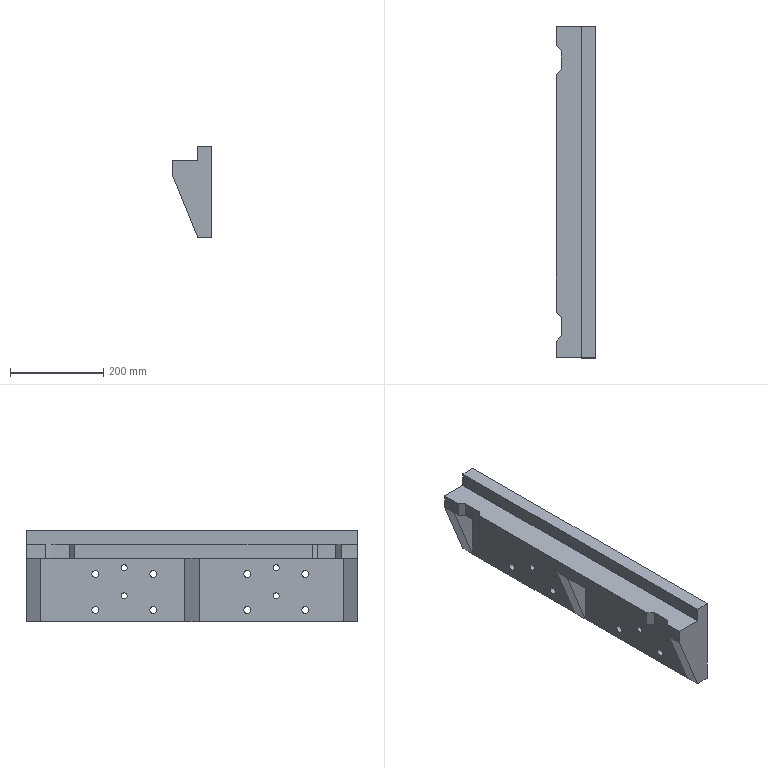Part | NX | features solid 2 | 1 solid | 39 faces | box 85 x 710 x 195 mm | volume 5567126 mm3 | plane 27 | cylinder 12 | commonest cylinder face diameters 15 x8 13 x4
STEP:
#1=CARTESIAN_POINT('',(780.,114.5,-108.));
#2=VERTEX_POINT('',#1);
#3=CARTESIAN_POINT('',(780.,107.,-108.));
#4=DIRECTION('',(1.,0.,0.));
#5=DIRECTION('',(0.,1.,0.));
#6=AXIS2_PLACEMENT_3D('',#3,#4,#5);
#7=CIRCLE('',#6,7.5);
#8=EDGE_CURVE('',#2,#2,#7,.F.);
#9=ORIENTED_EDGE('',*,*,#8,.F.);
#10=EDGE_LOOP('',(#9));
#11=FACE_BOUND('',#10,.T.);
#12=CARTESIAN_POINT('',(780.,114.5,-185.));
#13=VERTEX_POINT('',#12);
#14=CARTESIAN_POINT('',(780.,107.,-185.));
#15=DIRECTION('',(1.,0.,0.));
#16=DIRECTION('',(0.,1.,0.));
#17=AXIS2_PLACEMENT_3D('',#14,#15,#16);
#18=CIRCLE('',#17,7.5);
#19=EDGE_CURVE('',#13,#13,#18,.F.);
#20=ORIENTED_EDGE('',*,*,#19,.F.);
#21=EDGE_LOOP('',(#20));
#22=FACE_BOUND('',#21,.T.);
#23=CARTESIAN_POINT('',(780.,51.5,-155.));
#24=VERTEX_POINT('',#23);
#25=CARTESIAN_POINT('',(780.,45.,-155.));
#26=DIRECTION('',(1.,0.,0.));
#27=DIRECTION('',(0.,1.,0.));
#28=AXIS2_PLACEMENT_3D('',#25,#26,#27);
#29=CIRCLE('',#28,6.5);
#30=EDGE_CURVE('',#24,#24,#29,.T.);
#31=ORIENTED_EDGE('',*,*,#30,.T.);
#32=EDGE_LOOP('',(#31));
#33=FACE_BOUND('',#32,.T.);
#34=CARTESIAN_POINT('',(780.,-9.5,-185.));
#35=VERTEX_POINT('',#34);
#36=CARTESIAN_POINT('',(780.,-17.,-185.));
#37=DIRECTION('',(1.,0.,0.));
#38=DIRECTION('',(0.,1.,0.));
#39=AXIS2_PLACEMENT_3D('',#36,#37,#38);
#40=CIRCLE('',#39,7.5);
#41=EDGE_CURVE('',#35,#35,#40,.F.);
#42=ORIENTED_EDGE('',*,*,#41,.F.);
#43=EDGE_LOOP('',(#42));
#44=FACE_BOUND('',#43,.T.);
#45=CARTESIAN_POINT('',(780.,51.5,-95.));
#46=VERTEX_POINT('',#45);
#47=CARTESIAN_POINT('',(780.,45.,-95.));
#48=DIRECTION('',(1.,0.,0.));
#49=DIRECTION('',(0.,1.,0.));
#50=AXIS2_PLACEMENT_3D('',#47,#48,#49);
#51=CIRCLE('',#50,6.5);
#52=EDGE_CURVE('',#46,#46,#51,.T.);
#53=ORIENTED_EDGE('',*,*,#52,.T.);
#54=EDGE_LOOP('',(#53));
#55=FACE_BOUND('',#54,.T.);
#56=CARTESIAN_POINT('',(780.,-9.5,-108.));
#57=VERTEX_POINT('',#56);
#58=CARTESIAN_POINT('',(780.,-17.,-108.));
#59=DIRECTION('',(1.,0.,0.));
#60=DIRECTION('',(0.,1.,0.));
#61=AXIS2_PLACEMENT_3D('',#58,#59,#60);
#62=CIRCLE('',#61,7.5);
#63=EDGE_CURVE('',#57,#57,#62,.F.);
#64=ORIENTED_EDGE('',*,*,#63,.F.);
#65=EDGE_LOOP('',(#64));
#66=FACE_BOUND('',#65,.T.);
#67=CARTESIAN_POINT('',(780.,225.,-210.));
#68=VERTEX_POINT('',#67);
#69=CARTESIAN_POINT('',(780.,-85.,-210.));
#70=VERTEX_POINT('',#69);
#71=CARTESIAN_POINT('',(780.,-20.,-210.));
#72=DIRECTION('',(0.,1.,0.));
#73=VECTOR('',#72,1000.);
#74=LINE('',#71,#73);
#75=EDGE_CURVE('',#68,#70,#74,.F.);
#76=ORIENTED_EDGE('',*,*,#75,.T.);
#77=CARTESIAN_POINT('',(780.,-85.,-75.));
#78=VERTEX_POINT('',#77);
#79=CARTESIAN_POINT('',(780.,-85.,-75.));
#80=DIRECTION('',(0.,0.,-1.));
#81=VECTOR('',#80,1000.);
#82=LINE('',#79,#81);
#83=EDGE_CURVE('',#78,#70,#82,.T.);
#84=ORIENTED_EDGE('',*,*,#83,.F.);
#85=CARTESIAN_POINT('',(780.,225.,-75.));
#86=VERTEX_POINT('',#85);
#87=CARTESIAN_POINT('',(780.,-20.,-75.));
#88=DIRECTION('',(0.,1.,0.));
#89=VECTOR('',#88,1000.);
#90=LINE('',#87,#89);
#91=EDGE_CURVE('',#78,#86,#90,.T.);
#92=ORIENTED_EDGE('',*,*,#91,.T.);
#93=CARTESIAN_POINT('',(780.,225.,-75.));
#94=DIRECTION('',(0.,0.,-1.));
#95=VECTOR('',#94,1000.);
#96=LINE('',#93,#95);
#97=EDGE_CURVE('',#86,#68,#96,.T.);
#98=ORIENTED_EDGE('',*,*,#97,.T.);
#99=EDGE_LOOP('',(#76,#84,#92,#98));
#100=FACE_BOUND('',#99,.T.);
#101=CARTESIAN_POINT('',(780.,-330.,-15.974));
#102=DIRECTION('',(1.,0.,0.));
#103=DIRECTION('',(0.,1.,0.));
#104=AXIS2_PLACEMENT_3D('',#101,#102,#103);
#105=PLANE('',#104);
#106=ADVANCED_FACE('',(#11,#22,#33,#44,#55,#66,#100),#105,.F.);
#107=ORIENTED_EDGE('',*,*,#91,.F.);
#108=CARTESIAN_POINT('',(725.,-85.,-75.));
#109=VERTEX_POINT('',#108);
#110=CARTESIAN_POINT('',(780.,-85.,-75.));
#111=DIRECTION('',(-1.,0.,0.));
#112=VECTOR('',#111,1000.);
#113=LINE('',#110,#112);
#114=EDGE_CURVE('',#78,#109,#113,.T.);
#115=ORIENTED_EDGE('',*,*,#114,.T.);
#116=CARTESIAN_POINT('',(725.,151.,-75.));
#117=VERTEX_POINT('',#116);
#118=CARTESIAN_POINT('',(725.,-370.,-75.));
#119=DIRECTION('',(0.,-1.,0.));
#120=VECTOR('',#119,1000.);
#121=LINE('',#118,#120);
#122=EDGE_CURVE('',#117,#109,#121,.T.);
#123=ORIENTED_EDGE('',*,*,#122,.F.);
#124=CARTESIAN_POINT('',(736.,162.,-75.));
#125=VERTEX_POINT('',#124);
#126=CARTESIAN_POINT('',(842.,268.,-75.));
#127=DIRECTION('',(0.7071,0.7071,0.));
#128=VECTOR('',#127,1000.);
#129=LINE('',#126,#128);
#130=EDGE_CURVE('',#117,#125,#129,.T.);
#131=ORIENTED_EDGE('',*,*,#130,.T.);
#132=CARTESIAN_POINT('',(736.,202.,-75.));
#133=VERTEX_POINT('',#132);
#134=CARTESIAN_POINT('',(736.,330.,-75.));
#135=DIRECTION('',(0.,-1.,0.));
#136=VECTOR('',#135,1000.);
#137=LINE('',#134,#136);
#138=EDGE_CURVE('',#133,#125,#137,.T.);
#139=ORIENTED_EDGE('',*,*,#138,.F.);
#140=CARTESIAN_POINT('',(725.,213.,-75.));
#141=VERTEX_POINT('',#140);
#142=CARTESIAN_POINT('',(694.,244.,-75.));
#143=DIRECTION('',(-0.7071,0.7071,0.));
#144=VECTOR('',#143,1000.);
#145=LINE('',#142,#144);
#146=EDGE_CURVE('',#133,#141,#145,.T.);
#147=ORIENTED_EDGE('',*,*,#146,.T.);
#148=CARTESIAN_POINT('',(725.,225.,-75.));
#149=VERTEX_POINT('',#148);
#150=CARTESIAN_POINT('',(725.,-370.,-75.));
#151=DIRECTION('',(0.,-1.,0.));
#152=VECTOR('',#151,1000.);
#153=LINE('',#150,#152);
#154=EDGE_CURVE('',#149,#141,#153,.T.);
#155=ORIENTED_EDGE('',*,*,#154,.F.);
#156=CARTESIAN_POINT('',(780.,225.,-75.));
#157=DIRECTION('',(-1.,0.,0.));
#158=VECTOR('',#157,1000.);
#159=LINE('',#156,#158);
#160=EDGE_CURVE('',#86,#149,#159,.T.);
#161=ORIENTED_EDGE('',*,*,#160,.F.);
#162=EDGE_LOOP('',(#107,#115,#123,#131,#139,#147,#155,#161));
#163=FACE_BOUND('',#162,.T.);
#164=CARTESIAN_POINT('',(780.,330.,-75.));
#165=DIRECTION('',(0.,0.,1.));
#166=DIRECTION('',(0.,-1.,0.));
#167=AXIS2_PLACEMENT_3D('',#164,#165,#166);
#168=PLANE('',#167);
#169=ADVANCED_FACE('',(#163),#168,.F.);
#170=CARTESIAN_POINT('',(810.,255.,-15.));
#171=VERTEX_POINT('',#170);
#172=CARTESIAN_POINT('',(810.,-455.,-15.));
#173=VERTEX_POINT('',#172);
#174=CARTESIAN_POINT('',(810.,-185.,-15.));
#175=DIRECTION('',(0.,1.,0.));
#176=VECTOR('',#175,1000.);
#177=LINE('',#174,#176);
#178=EDGE_CURVE('',#171,#173,#177,.F.);
#179=ORIENTED_EDGE('',*,*,#178,.T.);
#180=CARTESIAN_POINT('',(810.,-455.,-210.));
#181=VERTEX_POINT('',#180);
#182=CARTESIAN_POINT('',(810.,-455.,-120.));
#183=DIRECTION('',(0.,0.,1.));
#184=VECTOR('',#183,1000.);
#185=LINE('',#182,#184);
#186=EDGE_CURVE('',#181,#173,#185,.T.);
#187=ORIENTED_EDGE('',*,*,#186,.F.);
#188=CARTESIAN_POINT('',(810.,255.,-210.));
#189=VERTEX_POINT('',#188);
#190=CARTESIAN_POINT('',(810.,-370.,-210.));
#191=DIRECTION('',(0.,1.,0.));
#192=VECTOR('',#191,1000.);
#193=LINE('',#190,#192);
#194=EDGE_CURVE('',#189,#181,#193,.F.);
#195=ORIENTED_EDGE('',*,*,#194,.F.);
#196=CARTESIAN_POINT('',(810.,255.,-0.4096));
#197=DIRECTION('',(0.,0.,-1.));
#198=VECTOR('',#197,1000.);
#199=LINE('',#196,#198);
#200=EDGE_CURVE('',#171,#189,#199,.T.);
#201=ORIENTED_EDGE('',*,*,#200,.F.);
#202=EDGE_LOOP('',(#179,#187,#195,#201));
#203=FACE_BOUND('',#202,.T.);
#204=CARTESIAN_POINT('',(810.,114.5,-108.));
#205=VERTEX_POINT('',#204);
#206=CARTESIAN_POINT('',(810.,107.,-108.));
#207=DIRECTION('',(1.,0.,0.));
#208=DIRECTION('',(0.,1.,0.));
#209=AXIS2_PLACEMENT_3D('',#206,#207,#208);
#210=CIRCLE('',#209,7.5);
#211=EDGE_CURVE('',#205,#205,#210,.F.);
#212=ORIENTED_EDGE('',*,*,#211,.T.);
#213=EDGE_LOOP('',(#212));
#214=FACE_BOUND('',#213,.T.);
#215=CARTESIAN_POINT('',(810.,114.5,-185.));
#216=VERTEX_POINT('',#215);
#217=CARTESIAN_POINT('',(810.,107.,-185.));
#218=DIRECTION('',(1.,0.,0.));
#219=DIRECTION('',(0.,1.,0.));
#220=AXIS2_PLACEMENT_3D('',#217,#218,#219);
#221=CIRCLE('',#220,7.5);
#222=EDGE_CURVE('',#216,#216,#221,.F.);
#223=ORIENTED_EDGE('',*,*,#222,.T.);
#224=EDGE_LOOP('',(#223));
#225=FACE_BOUND('',#224,.T.);
#226=CARTESIAN_POINT('',(810.,51.5,-155.));
#227=VERTEX_POINT('',#226);
#228=CARTESIAN_POINT('',(810.,45.,-155.));
#229=DIRECTION('',(1.,0.,0.));
#230=DIRECTION('',(0.,1.,0.));
#231=AXIS2_PLACEMENT_3D('',#228,#229,#230);
#232=CIRCLE('',#231,6.5);
#233=EDGE_CURVE('',#227,#227,#232,.T.);
#234=ORIENTED_EDGE('',*,*,#233,.F.);
#235=EDGE_LOOP('',(#234));
#236=FACE_BOUND('',#235,.T.);
#237=CARTESIAN_POINT('',(810.,-9.5,-185.));
#238=VERTEX_POINT('',#237);
#239=CARTESIAN_POINT('',(810.,-17.,-185.));
#240=DIRECTION('',(1.,0.,0.));
#241=DIRECTION('',(0.,1.,0.));
#242=AXIS2_PLACEMENT_3D('',#239,#240,#241);
#243=CIRCLE('',#242,7.5);
#244=EDGE_CURVE('',#238,#238,#243,.F.);
#245=ORIENTED_EDGE('',*,*,#244,.T.);
#246=EDGE_LOOP('',(#245));
#247=FACE_BOUND('',#246,.T.);
#248=CARTESIAN_POINT('',(810.,51.5,-95.));
#249=VERTEX_POINT('',#248);
#250=CARTESIAN_POINT('',(810.,45.,-95.));
#251=DIRECTION('',(1.,0.,0.));
#252=DIRECTION('',(0.,1.,0.));
#253=AXIS2_PLACEMENT_3D('',#250,#251,#252);
#254=CIRCLE('',#253,6.5);
#255=EDGE_CURVE('',#249,#249,#254,.T.);
#256=ORIENTED_EDGE('',*,*,#255,.F.);
#257=EDGE_LOOP('',(#256));
#258=FACE_BOUND('',#257,.T.);
#259=CARTESIAN_POINT('',(810.,-9.5,-108.));
#260=VERTEX_POINT('',#259);
#261=CARTESIAN_POINT('',(810.,-17.,-108.));
#262=DIRECTION('',(1.,0.,0.));
#263=DIRECTION('',(0.,1.,0.));
#264=AXIS2_PLACEMENT_3D('',#261,#262,#263);
#265=CIRCLE('',#264,7.5);
#266=EDGE_CURVE('',#260,#260,#265,.F.);
#267=ORIENTED_EDGE('',*,*,#266,.T.);
#268=EDGE_LOOP('',(#267));
#269=FACE_BOUND('',#268,.T.);
#270=CARTESIAN_POINT('',(810.,-210.5,-108.));
#271=VERTEX_POINT('',#270);
#272=CARTESIAN_POINT('',(810.,-218.,-108.));
#273=DIRECTION('',(1.,0.,0.));
#274=DIRECTION('',(0.,1.,0.));
#275=AXIS2_PLACEMENT_3D('',#272,#273,#274);
#276=CIRCLE('',#275,7.5);
#277=EDGE_CURVE('',#271,#271,#276,.F.);
#278=ORIENTED_EDGE('',*,*,#277,.T.);
#279=EDGE_LOOP('',(#278));
#280=FACE_BOUND('',#279,.T.);
#281=CARTESIAN_POINT('',(810.,-210.5,-185.));
#282=VERTEX_POINT('',#281);
#283=CARTESIAN_POINT('',(810.,-218.,-185.));
#284=DIRECTION('',(1.,0.,0.));
#285=DIRECTION('',(0.,1.,0.));
#286=AXIS2_PLACEMENT_3D('',#283,#284,#285);
#287=CIRCLE('',#286,7.5);
#288=EDGE_CURVE('',#282,#282,#287,.F.);
#289=ORIENTED_EDGE('',*,*,#288,.T.);
#290=EDGE_LOOP('',(#289));
#291=FACE_BOUND('',#290,.T.);
#292=CARTESIAN_POINT('',(810.,-273.5,-155.));
#293=VERTEX_POINT('',#292);
#294=CARTESIAN_POINT('',(810.,-280.,-155.));
#295=DIRECTION('',(1.,0.,0.));
#296=DIRECTION('',(0.,1.,0.));
#297=AXIS2_PLACEMENT_3D('',#294,#295,#296);
#298=CIRCLE('',#297,6.5);
#299=EDGE_CURVE('',#293,#293,#298,.T.);
#300=ORIENTED_EDGE('',*,*,#299,.F.);
#301=EDGE_LOOP('',(#300));
#302=FACE_BOUND('',#301,.T.);
#303=CARTESIAN_POINT('',(810.,-334.5,-185.));
#304=VERTEX_POINT('',#303);
#305=CARTESIAN_POINT('',(810.,-342.,-185.));
#306=DIRECTION('',(1.,0.,0.));
#307=DIRECTION('',(0.,1.,0.));
#308=AXIS2_PLACEMENT_3D('',#305,#306,#307);
#309=CIRCLE('',#308,7.5);
#310=EDGE_CURVE('',#304,#304,#309,.F.);
#311=ORIENTED_EDGE('',*,*,#310,.T.);
#312=EDGE_LOOP('',(#311));
#313=FACE_BOUND('',#312,.T.);
#314=CARTESIAN_POINT('',(810.,-273.5,-95.));
#315=VERTEX_POINT('',#314);
#316=CARTESIAN_POINT('',(810.,-280.,-95.));
#317=DIRECTION('',(1.,0.,0.));
#318=DIRECTION('',(0.,1.,0.));
#319=AXIS2_PLACEMENT_3D('',#316,#317,#318);
#320=CIRCLE('',#319,6.5);
#321=EDGE_CURVE('',#315,#315,#320,.T.);
#322=ORIENTED_EDGE('',*,*,#321,.F.);
#323=EDGE_LOOP('',(#322));
#324=FACE_BOUND('',#323,.T.);
#325=CARTESIAN_POINT('',(810.,-334.5,-108.));
#326=VERTEX_POINT('',#325);
#327=CARTESIAN_POINT('',(810.,-342.,-108.));
#328=DIRECTION('',(1.,0.,0.));
#329=DIRECTION('',(0.,1.,0.));
#330=AXIS2_PLACEMENT_3D('',#327,#328,#329);
#331=CIRCLE('',#330,7.5);
#332=EDGE_CURVE('',#326,#326,#331,.F.);
#333=ORIENTED_EDGE('',*,*,#332,.T.);
#334=EDGE_LOOP('',(#333));
#335=FACE_BOUND('',#334,.T.);
#336=CARTESIAN_POINT('',(810.,-370.,-15.974));
#337=DIRECTION('',(1.,0.,0.));
#338=DIRECTION('',(0.,1.,0.));
#339=AXIS2_PLACEMENT_3D('',#336,#337,#338);
#340=PLANE('',#339);
#341=ADVANCED_FACE('',(#203,#214,#225,#236,#247,#258,#269,#280,#291,#302,#313,#324,#335),#340,.T.);
#342=CARTESIAN_POINT('',(780.,255.,-210.));
#343=VERTEX_POINT('',#342);
#344=CARTESIAN_POINT('',(730.,255.,-210.));
#345=DIRECTION('',(-1.,0.,0.));
#346=VECTOR('',#345,1000.);
#347=LINE('',#344,#346);
#348=EDGE_CURVE('',#343,#189,#347,.F.);
#349=ORIENTED_EDGE('',*,*,#348,.T.);
#350=ORIENTED_EDGE('',*,*,#194,.T.);
#351=CARTESIAN_POINT('',(780.,-455.,-210.));
#352=VERTEX_POINT('',#351);
#353=CARTESIAN_POINT('',(830.,-455.,-210.));
#354=DIRECTION('',(1.,0.,0.));
#355=VECTOR('',#354,1000.);
#356=LINE('',#353,#355);
#357=EDGE_CURVE('',#181,#352,#356,.F.);
#358=ORIENTED_EDGE('',*,*,#357,.T.);
#359=CARTESIAN_POINT('',(780.,-425.,-210.));
#360=VERTEX_POINT('',#359);
#361=CARTESIAN_POINT('',(780.,-455.,-210.));
#362=DIRECTION('',(0.,-1.,0.));
#363=VECTOR('',#362,1000.);
#364=LINE('',#361,#363);
#365=EDGE_CURVE('',#360,#352,#364,.T.);
#366=ORIENTED_EDGE('',*,*,#365,.F.);
#367=CARTESIAN_POINT('',(780.,-115.,-210.));
#368=VERTEX_POINT('',#367);
#369=CARTESIAN_POINT('',(780.,-20.,-210.));
#370=DIRECTION('',(0.,1.,0.));
#371=VECTOR('',#370,1000.);
#372=LINE('',#369,#371);
#373=EDGE_CURVE('',#368,#360,#372,.F.);
#374=ORIENTED_EDGE('',*,*,#373,.F.);
#375=CARTESIAN_POINT('',(780.,-85.,-210.));
#376=DIRECTION('',(0.,-1.,0.));
#377=VECTOR('',#376,1000.);
#378=LINE('',#375,#377);
#379=EDGE_CURVE('',#70,#368,#378,.T.);
#380=ORIENTED_EDGE('',*,*,#379,.F.);
#381=ORIENTED_EDGE('',*,*,#75,.F.);
#382=CARTESIAN_POINT('',(780.,-20.,-210.));
#383=DIRECTION('',(0.,1.,0.));
#384=VECTOR('',#383,1000.);
#385=LINE('',#382,#384);
#386=EDGE_CURVE('',#343,#68,#385,.F.);
#387=ORIENTED_EDGE('',*,*,#386,.F.);
#388=EDGE_LOOP('',(#349,#350,#358,#366,#374,#380,#381,#387));
#389=FACE_BOUND('',#388,.T.);
#390=CARTESIAN_POINT('',(810.,-185.,-210.));
#391=DIRECTION('',(0.,0.,-1.));
#392=DIRECTION('',(1.,0.,0.));
#393=AXIS2_PLACEMENT_3D('',#390,#391,#392);
#394=PLANE('',#393);
#395=ADVANCED_FACE('',(#389),#394,.T.);
#396=ORIENTED_EDGE('',*,*,#211,.F.);
#397=EDGE_LOOP('',(#396));
#398=FACE_BOUND('',#397,.T.);
#399=ORIENTED_EDGE('',*,*,#8,.T.);
#400=EDGE_LOOP('',(#399));
#401=FACE_BOUND('',#400,.T.);
#402=CARTESIAN_POINT('',(910.,107.,-108.));
#403=DIRECTION('',(-1.,0.,0.));
#404=DIRECTION('',(0.,0.,-1.));
#405=AXIS2_PLACEMENT_3D('',#402,#403,#404);
#406=CYLINDRICAL_SURFACE('',#405,7.5);
#407=ADVANCED_FACE('',(#398,#401),#406,.F.);
#408=ORIENTED_EDGE('',*,*,#222,.F.);
#409=EDGE_LOOP('',(#408));
#410=FACE_BOUND('',#409,.T.);
#411=ORIENTED_EDGE('',*,*,#19,.T.);
#412=EDGE_LOOP('',(#411));
#413=FACE_BOUND('',#412,.T.);
#414=CARTESIAN_POINT('',(910.,107.,-185.));
#415=DIRECTION('',(-1.,0.,0.));
#416=DIRECTION('',(0.,0.,-1.));
#417=AXIS2_PLACEMENT_3D('',#414,#415,#416);
#418=CYLINDRICAL_SURFACE('',#417,7.5);
#419=ADVANCED_FACE('',(#410,#413),#418,.F.);
#420=ORIENTED_EDGE('',*,*,#233,.T.);
#421=EDGE_LOOP('',(#420));
#422=FACE_BOUND('',#421,.T.);
#423=ORIENTED_EDGE('',*,*,#30,.F.);
#424=EDGE_LOOP('',(#423));
#425=FACE_BOUND('',#424,.T.);
#426=CARTESIAN_POINT('',(910.,45.,-155.));
#427=DIRECTION('',(-1.,0.,0.));
#428=DIRECTION('',(0.,0.,-1.));
#429=AXIS2_PLACEMENT_3D('',#426,#427,#428);
#430=CYLINDRICAL_SURFACE('',#429,6.5);
#431=ADVANCED_FACE('',(#422,#425),#430,.F.);
#432=ORIENTED_EDGE('',*,*,#244,.F.);
#433=EDGE_LOOP('',(#432));
#434=FACE_BOUND('',#433,.T.);
#435=ORIENTED_EDGE('',*,*,#41,.T.);
#436=EDGE_LOOP('',(#435));
#437=FACE_BOUND('',#436,.T.);
#438=CARTESIAN_POINT('',(910.,-17.,-185.));
#439=DIRECTION('',(-1.,0.,0.));
#440=DIRECTION('',(0.,0.,-1.));
#441=AXIS2_PLACEMENT_3D('',#438,#439,#440);
#442=CYLINDRICAL_SURFACE('',#441,7.5);
#443=ADVANCED_FACE('',(#434,#437),#442,.F.);
#444=ORIENTED_EDGE('',*,*,#255,.T.);
#445=EDGE_LOOP('',(#444));
#446=FACE_BOUND('',#445,.T.);
#447=ORIENTED_EDGE('',*,*,#52,.F.);
#448=EDGE_LOOP('',(#447));
#449=FACE_BOUND('',#448,.T.);
#450=CARTESIAN_POINT('',(910.,45.,-95.));
#451=DIRECTION('',(-1.,0.,0.));
#452=DIRECTION('',(0.,0.,-1.));
#453=AXIS2_PLACEMENT_3D('',#450,#451,#452);
#454=CYLINDRICAL_SURFACE('',#453,6.5);
#455=ADVANCED_FACE('',(#446,#449),#454,.F.);
#456=ORIENTED_EDGE('',*,*,#266,.F.);
#457=EDGE_LOOP('',(#456));
#458=FACE_BOUND('',#457,.T.);
#459=ORIENTED_EDGE('',*,*,#63,.T.);
#460=EDGE_LOOP('',(#459));
#461=FACE_BOUND('',#460,.T.);
#462=CARTESIAN_POINT('',(910.,-17.,-108.));
#463=DIRECTION('',(-1.,0.,0.));
#464=DIRECTION('',(0.,0.,-1.));
#465=AXIS2_PLACEMENT_3D('',#462,#463,#464);
#466=CYLINDRICAL_SURFACE('',#465,7.5);
#467=ADVANCED_FACE('',(#458,#461),#466,.F.);
#468=ORIENTED_EDGE('',*,*,#332,.F.);
#469=EDGE_LOOP('',(#468));
#470=FACE_BOUND('',#469,.T.);
#471=CARTESIAN_POINT('',(780.,-334.5,-108.));
#472=VERTEX_POINT('',#471);
#473=CARTESIAN_POINT('',(780.,-342.,-108.));
#474=DIRECTION('',(1.,0.,0.));
#475=DIRECTION('',(0.,1.,0.));
#476=AXIS2_PLACEMENT_3D('',#473,#474,#475);
#477=CIRCLE('',#476,7.5);
#478=EDGE_CURVE('',#472,#472,#477,.F.);
#479=ORIENTED_EDGE('',*,*,#478,.T.);
#480=EDGE_LOOP('',(#479));
#481=FACE_BOUND('',#480,.T.);
#482=CARTESIAN_POINT('',(910.,-342.,-108.));
#483=DIRECTION('',(-1.,0.,0.));
#484=DIRECTION('',(0.,0.,-1.));
#485=AXIS2_PLACEMENT_3D('',#482,#483,#484);
#486=CYLINDRICAL_SURFACE('',#485,7.5);
#487=ADVANCED_FACE('',(#470,#481),#486,.F.);
#488=ORIENTED_EDGE('',*,*,#321,.T.);
#489=EDGE_LOOP('',(#488));
#490=FACE_BOUND('',#489,.T.);
#491=CARTESIAN_POINT('',(780.,-273.5,-95.));
#492=VERTEX_POINT('',#491);
#493=CARTESIAN_POINT('',(780.,-280.,-95.));
#494=DIRECTION('',(1.,0.,0.));
#495=DIRECTION('',(0.,1.,0.));
#496=AXIS2_PLACEMENT_3D('',#493,#494,#495);
#497=CIRCLE('',#496,6.5);
#498=EDGE_CURVE('',#492,#492,#497,.T.);
#499=ORIENTED_EDGE('',*,*,#498,.F.);
#500=EDGE_LOOP('',(#499));
#501=FACE_BOUND('',#500,.T.);
#502=CARTESIAN_POINT('',(910.,-280.,-95.));
#503=DIRECTION('',(-1.,0.,0.));
#504=DIRECTION('',(0.,0.,-1.));
#505=AXIS2_PLACEMENT_3D('',#502,#503,#504);
#506=CYLINDRICAL_SURFACE('',#505,6.5);
#507=ADVANCED_FACE('',(#490,#501),#506,.F.);
#508=ORIENTED_EDGE('',*,*,#310,.F.);
#509=EDGE_LOOP('',(#508));
#510=FACE_BOUND('',#509,.T.);
#511=CARTESIAN_POINT('',(780.,-334.5,-185.));
#512=VERTEX_POINT('',#511);
#513=CARTESIAN_POINT('',(780.,-342.,-185.));
#514=DIRECTION('',(1.,0.,0.));
#515=DIRECTION('',(0.,1.,0.));
#516=AXIS2_PLACEMENT_3D('',#513,#514,#515);
#517=CIRCLE('',#516,7.5);
#518=EDGE_CURVE('',#512,#512,#517,.F.);
#519=ORIENTED_EDGE('',*,*,#518,.T.);
#520=EDGE_LOOP('',(#519));
#521=FACE_BOUND('',#520,.T.);
#522=CARTESIAN_POINT('',(910.,-342.,-185.));
#523=DIRECTION('',(-1.,0.,0.));
#524=DIRECTION('',(0.,0.,-1.));
#525=AXIS2_PLACEMENT_3D('',#522,#523,#524);
#526=CYLINDRICAL_SURFACE('',#525,7.5);
#527=ADVANCED_FACE('',(#510,#521),#526,.F.);
#528=ORIENTED_EDGE('',*,*,#299,.T.);
#529=EDGE_LOOP('',(#528));
#530=FACE_BOUND('',#529,.T.);
#531=CARTESIAN_POINT('',(780.,-273.5,-155.));
#532=VERTEX_POINT('',#531);
#533=CARTESIAN_POINT('',(780.,-280.,-155.));
#534=DIRECTION('',(1.,0.,0.));
#535=DIRECTION('',(0.,1.,0.));
#536=AXIS2_PLACEMENT_3D('',#533,#534,#535);
#537=CIRCLE('',#536,6.5);
#538=EDGE_CURVE('',#532,#532,#537,.T.);
#539=ORIENTED_EDGE('',*,*,#538,.F.);
#540=EDGE_LOOP('',(#539));
#541=FACE_BOUND('',#540,.T.);
#542=CARTESIAN_POINT('',(910.,-280.,-155.));
#543=DIRECTION('',(-1.,0.,0.));
#544=DIRECTION('',(0.,0.,-1.));
#545=AXIS2_PLACEMENT_3D('',#542,#543,#544);
#546=CYLINDRICAL_SURFACE('',#545,6.5);
#547=ADVANCED_FACE('',(#530,#541),#546,.F.);
#548=ORIENTED_EDGE('',*,*,#288,.F.);
#549=EDGE_LOOP('',(#548));
#550=FACE_BOUND('',#549,.T.);
#551=CARTESIAN_POINT('',(780.,-210.5,-185.));
#552=VERTEX_POINT('',#551);
#553=CARTESIAN_POINT('',(780.,-218.,-185.));
#554=DIRECTION('',(1.,0.,0.));
#555=DIRECTION('',(0.,1.,0.));
#556=AXIS2_PLACEMENT_3D('',#553,#554,#555);
#557=CIRCLE('',#556,7.5);
#558=EDGE_CURVE('',#552,#552,#557,.F.);
#559=ORIENTED_EDGE('',*,*,#558,.T.);
#560=EDGE_LOOP('',(#559));
#561=FACE_BOUND('',#560,.T.);
#562=CARTESIAN_POINT('',(910.,-218.,-185.));
#563=DIRECTION('',(-1.,0.,0.));
#564=DIRECTION('',(0.,0.,-1.));
#565=AXIS2_PLACEMENT_3D('',#562,#563,#564);
#566=CYLINDRICAL_SURFACE('',#565,7.5);
#567=ADVANCED_FACE('',(#550,#561),#566,.F.);
#568=ORIENTED_EDGE('',*,*,#277,.F.);
#569=EDGE_LOOP('',(#568));
#570=FACE_BOUND('',#569,.T.);
#571=CARTESIAN_POINT('',(780.,-210.5,-108.));
#572=VERTEX_POINT('',#571);
#573=CARTESIAN_POINT('',(780.,-218.,-108.));
#574=DIRECTION('',(1.,0.,0.));
#575=DIRECTION('',(0.,1.,0.));
#576=AXIS2_PLACEMENT_3D('',#573,#574,#575);
#577=CIRCLE('',#576,7.5);
#578=EDGE_CURVE('',#572,#572,#577,.F.);
#579=ORIENTED_EDGE('',*,*,#578,.T.);
#580=EDGE_LOOP('',(#579));
#581=FACE_BOUND('',#580,.T.);
#582=CARTESIAN_POINT('',(910.,-218.,-108.));
#583=DIRECTION('',(-1.,0.,0.));
#584=DIRECTION('',(0.,0.,-1.));
#585=AXIS2_PLACEMENT_3D('',#582,#583,#584);
#586=CYLINDRICAL_SURFACE('',#585,7.5);
#587=ADVANCED_FACE('',(#570,#581),#586,.F.);
#588=ORIENTED_EDGE('',*,*,#478,.F.);
#589=EDGE_LOOP('',(#588));
#590=FACE_BOUND('',#589,.T.);
#591=ORIENTED_EDGE('',*,*,#498,.T.);
#592=EDGE_LOOP('',(#591));
#593=FACE_BOUND('',#592,.T.);
#594=ORIENTED_EDGE('',*,*,#518,.F.);
#595=EDGE_LOOP('',(#594));
#596=FACE_BOUND('',#595,.T.);
#597=ORIENTED_EDGE('',*,*,#538,.T.);
#598=EDGE_LOOP('',(#597));
#599=FACE_BOUND('',#598,.T.);
#600=ORIENTED_EDGE('',*,*,#558,.F.);
#601=EDGE_LOOP('',(#600));
#602=FACE_BOUND('',#601,.T.);
#603=ORIENTED_EDGE('',*,*,#578,.F.);
#604=EDGE_LOOP('',(#603));
#605=FACE_BOUND('',#604,.T.);
#606=ORIENTED_EDGE('',*,*,#373,.T.);
#607=CARTESIAN_POINT('',(780.,-425.,-75.));
#608=VERTEX_POINT('',#607);
#609=CARTESIAN_POINT('',(780.,-425.,-75.));
#610=DIRECTION('',(0.,0.,1.));
#611=VECTOR('',#610,1000.);
#612=LINE('',#609,#611);
#613=EDGE_CURVE('',#608,#360,#612,.F.);
#614=ORIENTED_EDGE('',*,*,#613,.F.);
#615=CARTESIAN_POINT('',(780.,-115.,-75.));
#616=VERTEX_POINT('',#615);
#617=CARTESIAN_POINT('',(780.,-20.,-75.));
#618=DIRECTION('',(0.,1.,0.));
#619=VECTOR('',#618,1000.);
#620=LINE('',#617,#619);
#621=EDGE_CURVE('',#608,#616,#620,.T.);
#622=ORIENTED_EDGE('',*,*,#621,.T.);
#623=CARTESIAN_POINT('',(780.,-115.,-75.));
#624=DIRECTION('',(0.,0.,-1.));
#625=VECTOR('',#624,1000.);
#626=LINE('',#623,#625);
#627=EDGE_CURVE('',#616,#368,#626,.T.);
#628=ORIENTED_EDGE('',*,*,#627,.T.);
#629=EDGE_LOOP('',(#606,#614,#622,#628));
#630=FACE_BOUND('',#629,.T.);
#631=CARTESIAN_POINT('',(780.,-330.,-15.974));
#632=DIRECTION('',(1.,0.,0.));
#633=DIRECTION('',(0.,1.,0.));
#634=AXIS2_PLACEMENT_3D('',#631,#632,#633);
#635=PLANE('',#634);
#636=ADVANCED_FACE('',(#590,#593,#596,#599,#602,#605,#630),#635,.F.);
#637=CARTESIAN_POINT('',(725.,-455.,-75.));
#638=VERTEX_POINT('',#637);
#639=CARTESIAN_POINT('',(755.671,-455.,-150.282));
#640=DIRECTION('',(-0.3773,0.,0.9261));
#641=VECTOR('',#640,1000.);
#642=LINE('',#639,#641);
#643=EDGE_CURVE('',#352,#638,#642,.T.);
#644=ORIENTED_EDGE('',*,*,#643,.F.);
#645=ORIENTED_EDGE('',*,*,#357,.F.);
#646=ORIENTED_EDGE('',*,*,#186,.T.);
#647=CARTESIAN_POINT('',(780.,-455.,-15.));
#648=VERTEX_POINT('',#647);
#649=CARTESIAN_POINT('',(830.,-455.,-15.));
#650=DIRECTION('',(-1.,0.,0.));
#651=VECTOR('',#650,1000.);
#652=LINE('',#649,#651);
#653=EDGE_CURVE('',#648,#173,#652,.F.);
#654=ORIENTED_EDGE('',*,*,#653,.F.);
#655=CARTESIAN_POINT('',(780.,-455.,-45.));
#656=VERTEX_POINT('',#655);
#657=CARTESIAN_POINT('',(780.,-455.,-120.));
#658=DIRECTION('',(0.,0.,1.));
#659=VECTOR('',#658,1000.);
#660=LINE('',#657,#659);
#661=EDGE_CURVE('',#656,#648,#660,.T.);
#662=ORIENTED_EDGE('',*,*,#661,.F.);
#663=CARTESIAN_POINT('',(725.,-455.,-45.));
#664=VERTEX_POINT('',#663);
#665=CARTESIAN_POINT('',(830.,-455.,-45.));
#666=DIRECTION('',(-1.,0.,0.));
#667=VECTOR('',#666,1000.);
#668=LINE('',#665,#667);
#669=EDGE_CURVE('',#664,#656,#668,.F.);
#670=ORIENTED_EDGE('',*,*,#669,.F.);
#671=CARTESIAN_POINT('',(725.,-455.,-120.));
#672=DIRECTION('',(0.,0.,1.));
#673=VECTOR('',#672,1000.);
#674=LINE('',#671,#673);
#675=EDGE_CURVE('',#638,#664,#674,.T.);
#676=ORIENTED_EDGE('',*,*,#675,.F.);
#677=EDGE_LOOP('',(#644,#645,#646,#654,#662,#670,#676));
#678=FACE_BOUND('',#677,.T.);
#679=CARTESIAN_POINT('',(830.,-455.,-120.));
#680=DIRECTION('',(0.,-1.,0.));
#681=DIRECTION('',(0.,0.,-1.));
#682=AXIS2_PLACEMENT_3D('',#679,#680,#681);
#683=PLANE('',#682);
#684=ADVANCED_FACE('',(#678),#683,.T.);
#685=ORIENTED_EDGE('',*,*,#348,.F.);
#686=CARTESIAN_POINT('',(725.,255.,-75.));
#687=VERTEX_POINT('',#686);
#688=CARTESIAN_POINT('',(732.829,255.,-94.218));
#689=DIRECTION('',(0.3773,0.,-0.9261));
#690=VECTOR('',#689,1000.);
#691=LINE('',#688,#690);
#692=EDGE_CURVE('',#687,#343,#691,.T.);
#693=ORIENTED_EDGE('',*,*,#692,.F.);
#694=CARTESIAN_POINT('',(725.,255.,-45.));
#695=VERTEX_POINT('',#694);
#696=CARTESIAN_POINT('',(725.,255.,-0.4096));
#697=DIRECTION('',(0.,0.,-1.));
#698=VECTOR('',#697,1000.);
#699=LINE('',#696,#698);
#700=EDGE_CURVE('',#695,#687,#699,.T.);
#701=ORIENTED_EDGE('',*,*,#700,.F.);
#702=CARTESIAN_POINT('',(780.,255.,-45.));
#703=VERTEX_POINT('',#702);
#704=CARTESIAN_POINT('',(730.,255.,-45.));
#705=DIRECTION('',(1.,0.,0.));
#706=VECTOR('',#705,1000.);
#707=LINE('',#704,#706);
#708=EDGE_CURVE('',#703,#695,#707,.F.);
#709=ORIENTED_EDGE('',*,*,#708,.F.);
#710=CARTESIAN_POINT('',(780.,255.,-15.));
#711=VERTEX_POINT('',#710);
#712=CARTESIAN_POINT('',(780.,255.,-0.4096));
#713=DIRECTION('',(0.,0.,-1.));
#714=VECTOR('',#713,1000.);
#715=LINE('',#712,#714);
#716=EDGE_CURVE('',#711,#703,#715,.T.);
#717=ORIENTED_EDGE('',*,*,#716,.F.);
#718=CARTESIAN_POINT('',(730.,255.,-15.));
#719=DIRECTION('',(1.,0.,0.));
#720=VECTOR('',#719,1000.);
#721=LINE('',#718,#720);
#722=EDGE_CURVE('',#171,#711,#721,.F.);
#723=ORIENTED_EDGE('',*,*,#722,.F.);
#724=ORIENTED_EDGE('',*,*,#200,.T.);
#725=EDGE_LOOP('',(#685,#693,#701,#709,#717,#723,#724));
#726=FACE_BOUND('',#725,.T.);
#727=CARTESIAN_POINT('',(730.,255.,-0.4096));
#728=DIRECTION('',(0.,1.,0.));
#729=DIRECTION('',(0.,0.,1.));
#730=AXIS2_PLACEMENT_3D('',#727,#728,#729);
#731=PLANE('',#730);
#732=ADVANCED_FACE('',(#726),#731,.T.);
#733=CARTESIAN_POINT('',(725.,151.,-45.));
#734=VERTEX_POINT('',#733);
#735=CARTESIAN_POINT('',(725.,-357.,-45.));
#736=VERTEX_POINT('',#735);
#737=CARTESIAN_POINT('',(725.,-20.,-45.));
#738=DIRECTION('',(0.,1.,0.));
#739=VECTOR('',#738,1000.);
#740=LINE('',#737,#739);
#741=EDGE_CURVE('',#734,#736,#740,.F.);
#742=ORIENTED_EDGE('',*,*,#741,.F.);
#743=CARTESIAN_POINT('',(725.,151.,-55.974));
#744=DIRECTION('',(0.,0.,-1.));
#745=VECTOR('',#744,1000.);
#746=LINE('',#743,#745);
#747=EDGE_CURVE('',#734,#117,#746,.T.);
#748=ORIENTED_EDGE('',*,*,#747,.T.);
#749=ORIENTED_EDGE('',*,*,#122,.T.);
#750=CARTESIAN_POINT('',(725.,-115.,-75.));
#751=VERTEX_POINT('',#750);
#752=CARTESIAN_POINT('',(725.,-85.,-75.));
#753=DIRECTION('',(0.,-1.,0.));
#754=VECTOR('',#753,1000.);
#755=LINE('',#752,#754);
#756=EDGE_CURVE('',#109,#751,#755,.T.);
#757=ORIENTED_EDGE('',*,*,#756,.T.);
#758=CARTESIAN_POINT('',(725.,-357.,-75.));
#759=VERTEX_POINT('',#758);
#760=CARTESIAN_POINT('',(725.,-370.,-75.));
#761=DIRECTION('',(0.,-1.,0.));
#762=VECTOR('',#761,1000.);
#763=LINE('',#760,#762);
#764=EDGE_CURVE('',#751,#759,#763,.T.);
#765=ORIENTED_EDGE('',*,*,#764,.T.);
#766=CARTESIAN_POINT('',(725.,-357.,-55.974));
#767=DIRECTION('',(0.,0.,1.));
#768=VECTOR('',#767,1000.);
#769=LINE('',#766,#768);
#770=EDGE_CURVE('',#759,#736,#769,.T.);
#771=ORIENTED_EDGE('',*,*,#770,.T.);
#772=EDGE_LOOP('',(#742,#748,#749,#757,#765,#771));
#773=FACE_BOUND('',#772,.T.);
#774=CARTESIAN_POINT('',(725.,-370.,-55.974));
#775=DIRECTION('',(1.,0.,0.));
#776=DIRECTION('',(0.,1.,0.));
#777=AXIS2_PLACEMENT_3D('',#774,#775,#776);
#778=PLANE('',#777);
#779=ADVANCED_FACE('',(#773),#778,.F.);
#780=CARTESIAN_POINT('',(725.,-419.,-45.));
#781=VERTEX_POINT('',#780);
#782=CARTESIAN_POINT('',(725.,-20.,-45.));
#783=DIRECTION('',(0.,1.,0.));
#784=VECTOR('',#783,1000.);
#785=LINE('',#782,#784);
#786=EDGE_CURVE('',#781,#664,#785,.F.);
#787=ORIENTED_EDGE('',*,*,#786,.F.);
#788=CARTESIAN_POINT('',(725.,-419.,-75.));
#789=VERTEX_POINT('',#788);
#790=CARTESIAN_POINT('',(725.,-419.,-55.974));
#791=DIRECTION('',(0.,0.,-1.));
#792=VECTOR('',#791,1000.);
#793=LINE('',#790,#792);
#794=EDGE_CURVE('',#781,#789,#793,.T.);
#795=ORIENTED_EDGE('',*,*,#794,.T.);
#796=CARTESIAN_POINT('',(725.,-425.,-75.));
#797=VERTEX_POINT('',#796);
#798=CARTESIAN_POINT('',(725.,-370.,-75.));
#799=DIRECTION('',(0.,-1.,0.));
#800=VECTOR('',#799,1000.);
#801=LINE('',#798,#800);
#802=EDGE_CURVE('',#789,#797,#801,.T.);
#803=ORIENTED_EDGE('',*,*,#802,.T.);
#804=CARTESIAN_POINT('',(725.,-455.,-75.));
#805=DIRECTION('',(0.,-1.,0.));
#806=VECTOR('',#805,1000.);
#807=LINE('',#804,#806);
#808=EDGE_CURVE('',#797,#638,#807,.T.);
#809=ORIENTED_EDGE('',*,*,#808,.T.);
#810=ORIENTED_EDGE('',*,*,#675,.T.);
#811=EDGE_LOOP('',(#787,#795,#803,#809,#810));
#812=FACE_BOUND('',#811,.T.);
#813=CARTESIAN_POINT('',(725.,-370.,-55.974));
#814=DIRECTION('',(1.,0.,0.));
#815=DIRECTION('',(0.,1.,0.));
#816=AXIS2_PLACEMENT_3D('',#813,#814,#815);
#817=PLANE('',#816);
#818=ADVANCED_FACE('',(#812),#817,.F.);
#819=ORIENTED_EDGE('',*,*,#722,.T.);
#820=CARTESIAN_POINT('',(780.,-185.,-15.));
#821=DIRECTION('',(0.,1.,0.));
#822=VECTOR('',#821,1000.);
#823=LINE('',#820,#822);
#824=EDGE_CURVE('',#711,#648,#823,.F.);
#825=ORIENTED_EDGE('',*,*,#824,.T.);
#826=ORIENTED_EDGE('',*,*,#653,.T.);
#827=ORIENTED_EDGE('',*,*,#178,.F.);
#828=EDGE_LOOP('',(#819,#825,#826,#827));
#829=FACE_BOUND('',#828,.T.);
#830=CARTESIAN_POINT('',(885.,-185.,-15.));
#831=DIRECTION('',(0.,0.,1.));
#832=DIRECTION('',(-1.,0.,0.));
#833=AXIS2_PLACEMENT_3D('',#830,#831,#832);
#834=PLANE('',#833);
#835=ADVANCED_FACE('',(#829),#834,.T.);
#836=ORIENTED_EDGE('',*,*,#716,.T.);
#837=CARTESIAN_POINT('',(780.,-20.,-45.));
#838=DIRECTION('',(0.,1.,0.));
#839=VECTOR('',#838,1000.);
#840=LINE('',#837,#839);
#841=EDGE_CURVE('',#703,#656,#840,.F.);
#842=ORIENTED_EDGE('',*,*,#841,.T.);
#843=ORIENTED_EDGE('',*,*,#661,.T.);
#844=ORIENTED_EDGE('',*,*,#824,.F.);
#845=EDGE_LOOP('',(#836,#842,#843,#844));
#846=FACE_BOUND('',#845,.T.);
#847=CARTESIAN_POINT('',(780.,-370.,-15.974));
#848=DIRECTION('',(1.,0.,0.));
#849=DIRECTION('',(0.,1.,0.));
#850=AXIS2_PLACEMENT_3D('',#847,#848,#849);
#851=PLANE('',#850);
#852=ADVANCED_FACE('',(#846),#851,.F.);
#853=CARTESIAN_POINT('',(736.,162.,-45.));
#854=VERTEX_POINT('',#853);
#855=CARTESIAN_POINT('',(736.,202.,-45.));
#856=VERTEX_POINT('',#855);
#857=CARTESIAN_POINT('',(736.,-20.,-45.));
#858=DIRECTION('',(0.,-1.,0.));
#859=VECTOR('',#858,1000.);
#860=LINE('',#857,#859);
#861=EDGE_CURVE('',#854,#856,#860,.F.);
#862=ORIENTED_EDGE('',*,*,#861,.F.);
#863=CARTESIAN_POINT('',(667.,93.,-45.));
#864=DIRECTION('',(0.7071,0.7071,0.));
#865=VECTOR('',#864,1000.);
#866=LINE('',#863,#865);
#867=EDGE_CURVE('',#854,#734,#866,.F.);
#868=ORIENTED_EDGE('',*,*,#867,.T.);
#869=ORIENTED_EDGE('',*,*,#741,.T.);
#870=CARTESIAN_POINT('',(736.,-368.,-45.));
#871=VERTEX_POINT('',#870);
#872=CARTESIAN_POINT('',(584.,-216.,-45.));
#873=DIRECTION('',(-0.7071,0.7071,0.));
#874=VECTOR('',#873,1000.);
#875=LINE('',#872,#874);
#876=EDGE_CURVE('',#736,#871,#875,.F.);
#877=ORIENTED_EDGE('',*,*,#876,.T.);
#878=CARTESIAN_POINT('',(736.,-408.,-45.));
#879=VERTEX_POINT('',#878);
#880=CARTESIAN_POINT('',(736.,-20.,-45.));
#881=DIRECTION('',(0.,-1.,0.));
#882=VECTOR('',#881,1000.);
#883=LINE('',#880,#882);
#884=EDGE_CURVE('',#879,#871,#883,.F.);
#885=ORIENTED_EDGE('',*,*,#884,.F.);
#886=CARTESIAN_POINT('',(952.,-192.,-45.));
#887=DIRECTION('',(0.7071,0.7071,0.));
#888=VECTOR('',#887,1000.);
#889=LINE('',#886,#888);
#890=EDGE_CURVE('',#879,#781,#889,.F.);
#891=ORIENTED_EDGE('',*,*,#890,.T.);
#892=ORIENTED_EDGE('',*,*,#786,.T.);
#893=ORIENTED_EDGE('',*,*,#669,.T.);
#894=ORIENTED_EDGE('',*,*,#841,.F.);
#895=ORIENTED_EDGE('',*,*,#708,.T.);
#896=CARTESIAN_POINT('',(725.,213.,-45.));
#897=VERTEX_POINT('',#896);
#898=CARTESIAN_POINT('',(725.,-20.,-45.));
#899=DIRECTION('',(0.,1.,0.));
#900=VECTOR('',#899,1000.);
#901=LINE('',#898,#900);
#902=EDGE_CURVE('',#695,#897,#901,.F.);
#903=ORIENTED_EDGE('',*,*,#902,.T.);
#904=CARTESIAN_POINT('',(869.,69.,-45.));
#905=DIRECTION('',(-0.7071,0.7071,0.));
#906=VECTOR('',#905,1000.);
#907=LINE('',#904,#906);
#908=EDGE_CURVE('',#897,#856,#907,.F.);
#909=ORIENTED_EDGE('',*,*,#908,.T.);
#910=EDGE_LOOP('',(#862,#868,#869,#877,#885,#891,#892,#893,#894,#895,#903,#909));
#911=FACE_BOUND('',#910,.T.);
#912=CARTESIAN_POINT('',(780.,-20.,-45.));
#913=DIRECTION('',(0.,0.,1.));
#914=DIRECTION('',(0.,-1.,0.));
#915=AXIS2_PLACEMENT_3D('',#912,#913,#914);
#916=PLANE('',#915);
#917=ADVANCED_FACE('',(#911),#916,.T.);
#918=ORIENTED_EDGE('',*,*,#621,.F.);
#919=CARTESIAN_POINT('',(780.,-425.,-75.));
#920=DIRECTION('',(-1.,0.,0.));
#921=VECTOR('',#920,1000.);
#922=LINE('',#919,#921);
#923=EDGE_CURVE('',#608,#797,#922,.T.);
#924=ORIENTED_EDGE('',*,*,#923,.T.);
#925=ORIENTED_EDGE('',*,*,#802,.F.);
#926=CARTESIAN_POINT('',(736.,-408.,-75.));
#927=VERTEX_POINT('',#926);
#928=CARTESIAN_POINT('',(1127.,-17.,-75.));
#929=DIRECTION('',(0.7071,0.7071,0.));
#930=VECTOR('',#929,1000.);
#931=LINE('',#928,#930);
#932=EDGE_CURVE('',#789,#927,#931,.T.);
#933=ORIENTED_EDGE('',*,*,#932,.T.);
#934=CARTESIAN_POINT('',(736.,-368.,-75.));
#935=VERTEX_POINT('',#934);
#936=CARTESIAN_POINT('',(736.,330.,-75.));
#937=DIRECTION('',(0.,-1.,0.));
#938=VECTOR('',#937,1000.);
#939=LINE('',#936,#938);
#940=EDGE_CURVE('',#935,#927,#939,.T.);
#941=ORIENTED_EDGE('',*,*,#940,.F.);
#942=CARTESIAN_POINT('',(409.,-41.,-75.));
#943=DIRECTION('',(-0.7071,0.7071,0.));
#944=VECTOR('',#943,1000.);
#945=LINE('',#942,#944);
#946=EDGE_CURVE('',#935,#759,#945,.T.);
#947=ORIENTED_EDGE('',*,*,#946,.T.);
#948=ORIENTED_EDGE('',*,*,#764,.F.);
#949=CARTESIAN_POINT('',(780.,-115.,-75.));
#950=DIRECTION('',(-1.,0.,0.));
#951=VECTOR('',#950,1000.);
#952=LINE('',#949,#951);
#953=EDGE_CURVE('',#616,#751,#952,.T.);
#954=ORIENTED_EDGE('',*,*,#953,.F.);
#955=EDGE_LOOP('',(#918,#924,#925,#933,#941,#947,#948,#954));
#956=FACE_BOUND('',#955,.T.);
#957=CARTESIAN_POINT('',(780.,330.,-75.));
#958=DIRECTION('',(0.,0.,1.));
#959=DIRECTION('',(0.,-1.,0.));
#960=AXIS2_PLACEMENT_3D('',#957,#958,#959);
#961=PLANE('',#960);
#962=ADVANCED_FACE('',(#956),#961,.F.);
#963=CARTESIAN_POINT('',(725.,-370.,-75.));
#964=DIRECTION('',(0.,-1.,0.));
#965=VECTOR('',#964,1000.);
#966=LINE('',#963,#965);
#967=EDGE_CURVE('',#687,#149,#966,.T.);
#968=ORIENTED_EDGE('',*,*,#967,.T.);
#969=ORIENTED_EDGE('',*,*,#154,.T.);
#970=CARTESIAN_POINT('',(725.,213.,-55.974));
#971=DIRECTION('',(0.,0.,1.));
#972=VECTOR('',#971,1000.);
#973=LINE('',#970,#972);
#974=EDGE_CURVE('',#141,#897,#973,.T.);
#975=ORIENTED_EDGE('',*,*,#974,.T.);
#976=ORIENTED_EDGE('',*,*,#902,.F.);
#977=ORIENTED_EDGE('',*,*,#700,.T.);
#978=EDGE_LOOP('',(#968,#969,#975,#976,#977));
#979=FACE_BOUND('',#978,.T.);
#980=CARTESIAN_POINT('',(725.,-370.,-55.974));
#981=DIRECTION('',(1.,0.,0.));
#982=DIRECTION('',(0.,1.,0.));
#983=AXIS2_PLACEMENT_3D('',#980,#981,#982);
#984=PLANE('',#983);
#985=ADVANCED_FACE('',(#979),#984,.F.);
#986=ORIENTED_EDGE('',*,*,#884,.T.);
#987=CARTESIAN_POINT('',(736.,-368.,-25.));
#988=DIRECTION('',(0.,0.,-1.));
#989=VECTOR('',#988,1000.);
#990=LINE('',#987,#989);
#991=EDGE_CURVE('',#871,#935,#990,.T.);
#992=ORIENTED_EDGE('',*,*,#991,.T.);
#993=ORIENTED_EDGE('',*,*,#940,.T.);
#994=CARTESIAN_POINT('',(736.,-408.,-25.));
#995=DIRECTION('',(0.,0.,-1.));
#996=VECTOR('',#995,1000.);
#997=LINE('',#994,#996);
#998=EDGE_CURVE('',#879,#927,#997,.T.);
#999=ORIENTED_EDGE('',*,*,#998,.F.);
#1000=EDGE_LOOP('',(#986,#992,#993,#999));
#1001=FACE_BOUND('',#1000,.T.);
#1002=CARTESIAN_POINT('',(736.,-408.,-25.));
#1003=DIRECTION('',(-1.,0.,0.));
#1004=DIRECTION('',(0.,0.,1.));
#1005=AXIS2_PLACEMENT_3D('',#1002,#1003,#1004);
#1006=PLANE('',#1005);
#1007=ADVANCED_FACE('',(#1001),#1006,.T.);
#1008=ORIENTED_EDGE('',*,*,#998,.T.);
#1009=ORIENTED_EDGE('',*,*,#932,.F.);
#1010=ORIENTED_EDGE('',*,*,#794,.F.);
#1011=ORIENTED_EDGE('',*,*,#890,.F.);
#1012=EDGE_LOOP('',(#1008,#1009,#1010,#1011));
#1013=FACE_BOUND('',#1012,.T.);
#1014=CARTESIAN_POINT('',(736.,-408.,-25.));
#1015=DIRECTION('',(0.7071,-0.7071,0.));
#1016=DIRECTION('',(0.7071,0.7071,0.));
#1017=AXIS2_PLACEMENT_3D('',#1014,#1015,#1016);
#1018=PLANE('',#1017);
#1019=ADVANCED_FACE('',(#1013),#1018,.F.);
#1020=ORIENTED_EDGE('',*,*,#770,.F.);
#1021=ORIENTED_EDGE('',*,*,#946,.F.);
#1022=ORIENTED_EDGE('',*,*,#991,.F.);
#1023=ORIENTED_EDGE('',*,*,#876,.F.);
#1024=EDGE_LOOP('',(#1020,#1021,#1022,#1023));
#1025=FACE_BOUND('',#1024,.T.);
#1026=CARTESIAN_POINT('',(724.,-356.,-25.));
#1027=DIRECTION('',(0.7071,0.7071,0.));
#1028=DIRECTION('',(-0.7071,0.7071,0.));
#1029=AXIS2_PLACEMENT_3D('',#1026,#1027,#1028);
#1030=PLANE('',#1029);
#1031=ADVANCED_FACE('',(#1025),#1030,.F.);
#1032=ORIENTED_EDGE('',*,*,#861,.T.);
#1033=CARTESIAN_POINT('',(736.,202.,-25.));
#1034=DIRECTION('',(0.,0.,-1.));
#1035=VECTOR('',#1034,1000.);
#1036=LINE('',#1033,#1035);
#1037=EDGE_CURVE('',#856,#133,#1036,.T.);
#1038=ORIENTED_EDGE('',*,*,#1037,.T.);
#1039=ORIENTED_EDGE('',*,*,#138,.T.);
#1040=CARTESIAN_POINT('',(736.,162.,-25.));
#1041=DIRECTION('',(0.,0.,-1.));
#1042=VECTOR('',#1041,1000.);
#1043=LINE('',#1040,#1042);
#1044=EDGE_CURVE('',#854,#125,#1043,.T.);
#1045=ORIENTED_EDGE('',*,*,#1044,.F.);
#1046=EDGE_LOOP('',(#1032,#1038,#1039,#1045));
#1047=FACE_BOUND('',#1046,.T.);
#1048=CARTESIAN_POINT('',(736.,162.,-25.));
#1049=DIRECTION('',(-1.,0.,0.));
#1050=DIRECTION('',(0.,0.,1.));
#1051=AXIS2_PLACEMENT_3D('',#1048,#1049,#1050);
#1052=PLANE('',#1051);
#1053=ADVANCED_FACE('',(#1047),#1052,.T.);
#1054=ORIENTED_EDGE('',*,*,#1044,.T.);
#1055=ORIENTED_EDGE('',*,*,#130,.F.);
#1056=ORIENTED_EDGE('',*,*,#747,.F.);
#1057=ORIENTED_EDGE('',*,*,#867,.F.);
#1058=EDGE_LOOP('',(#1054,#1055,#1056,#1057));
#1059=FACE_BOUND('',#1058,.T.);
#1060=CARTESIAN_POINT('',(736.,162.,-25.));
#1061=DIRECTION('',(0.7071,-0.7071,0.));
#1062=DIRECTION('',(0.7071,0.7071,0.));
#1063=AXIS2_PLACEMENT_3D('',#1060,#1061,#1062);
#1064=PLANE('',#1063);
#1065=ADVANCED_FACE('',(#1059),#1064,.F.);
#1066=ORIENTED_EDGE('',*,*,#974,.F.);
#1067=ORIENTED_EDGE('',*,*,#146,.F.);
#1068=ORIENTED_EDGE('',*,*,#1037,.F.);
#1069=ORIENTED_EDGE('',*,*,#908,.F.);
#1070=EDGE_LOOP('',(#1066,#1067,#1068,#1069));
#1071=FACE_BOUND('',#1070,.T.);
#1072=CARTESIAN_POINT('',(724.,214.,-25.));
#1073=DIRECTION('',(0.7071,0.7071,0.));
#1074=DIRECTION('',(-0.7071,0.7071,0.));
#1075=AXIS2_PLACEMENT_3D('',#1072,#1073,#1074);
#1076=PLANE('',#1075);
#1077=ADVANCED_FACE('',(#1071),#1076,.F.);
#1078=CARTESIAN_POINT('',(732.829,225.,-94.218));
#1079=DIRECTION('',(0.3773,0.,-0.9261));
#1080=VECTOR('',#1079,1000.);
#1081=LINE('',#1078,#1080);
#1082=EDGE_CURVE('',#68,#149,#1081,.F.);
#1083=ORIENTED_EDGE('',*,*,#1082,.F.);
#1084=ORIENTED_EDGE('',*,*,#97,.F.);
#1085=ORIENTED_EDGE('',*,*,#160,.T.);
#1086=EDGE_LOOP('',(#1083,#1084,#1085));
#1087=FACE_BOUND('',#1086,.T.);
#1088=CARTESIAN_POINT('',(780.,225.,-75.));
#1089=DIRECTION('',(0.,1.,0.));
#1090=DIRECTION('',(-1.,0.,0.));
#1091=AXIS2_PLACEMENT_3D('',#1088,#1089,#1090);
#1092=PLANE('',#1091);
#1093=ADVANCED_FACE('',(#1087),#1092,.F.);
#1094=ORIENTED_EDGE('',*,*,#967,.F.);
#1095=ORIENTED_EDGE('',*,*,#692,.T.);
#1096=ORIENTED_EDGE('',*,*,#386,.T.);
#1097=ORIENTED_EDGE('',*,*,#1082,.T.);
#1098=EDGE_LOOP('',(#1094,#1095,#1096,#1097));
#1099=FACE_BOUND('',#1098,.T.);
#1100=CARTESIAN_POINT('',(725.,255.,-75.));
#1101=DIRECTION('',(0.9261,0.,0.3773));
#1102=DIRECTION('',(0.3773,0.,-0.9261));
#1103=AXIS2_PLACEMENT_3D('',#1100,#1101,#1102);
#1104=PLANE('',#1103);
#1105=ADVANCED_FACE('',(#1099),#1104,.F.);
#1106=CARTESIAN_POINT('',(732.829,-85.,-94.218));
#1107=DIRECTION('',(0.3773,0.,-0.9261));
#1108=VECTOR('',#1107,1000.);
#1109=LINE('',#1106,#1108);
#1110=EDGE_CURVE('',#109,#70,#1109,.T.);
#1111=ORIENTED_EDGE('',*,*,#1110,.F.);
#1112=ORIENTED_EDGE('',*,*,#114,.F.);
#1113=ORIENTED_EDGE('',*,*,#83,.T.);
#1114=EDGE_LOOP('',(#1111,#1112,#1113));
#1115=FACE_BOUND('',#1114,.T.);
#1116=CARTESIAN_POINT('',(780.,-85.,-75.));
#1117=DIRECTION('',(0.,1.,0.));
#1118=DIRECTION('',(-1.,0.,0.));
#1119=AXIS2_PLACEMENT_3D('',#1116,#1117,#1118);
#1120=PLANE('',#1119);
#1121=ADVANCED_FACE('',(#1115),#1120,.T.);
#1122=CARTESIAN_POINT('',(732.829,-115.,-94.218));
#1123=DIRECTION('',(0.3773,0.,-0.9261));
#1124=VECTOR('',#1123,1000.);
#1125=LINE('',#1122,#1124);
#1126=EDGE_CURVE('',#368,#751,#1125,.F.);
#1127=ORIENTED_EDGE('',*,*,#1126,.F.);
#1128=ORIENTED_EDGE('',*,*,#627,.F.);
#1129=ORIENTED_EDGE('',*,*,#953,.T.);
#1130=EDGE_LOOP('',(#1127,#1128,#1129));
#1131=FACE_BOUND('',#1130,.T.);
#1132=CARTESIAN_POINT('',(780.,-115.,-75.));
#1133=DIRECTION('',(0.,1.,0.));
#1134=DIRECTION('',(-1.,0.,0.));
#1135=AXIS2_PLACEMENT_3D('',#1132,#1133,#1134);
#1136=PLANE('',#1135);
#1137=ADVANCED_FACE('',(#1131),#1136,.F.);
#1138=ORIENTED_EDGE('',*,*,#756,.F.);
#1139=ORIENTED_EDGE('',*,*,#1110,.T.);
#1140=ORIENTED_EDGE('',*,*,#379,.T.);
#1141=ORIENTED_EDGE('',*,*,#1126,.T.);
#1142=EDGE_LOOP('',(#1138,#1139,#1140,#1141));
#1143=FACE_BOUND('',#1142,.T.);
#1144=CARTESIAN_POINT('',(725.,-85.,-75.));
#1145=DIRECTION('',(0.9261,0.,0.3773));
#1146=DIRECTION('',(0.3773,0.,-0.9261));
#1147=AXIS2_PLACEMENT_3D('',#1144,#1145,#1146);
#1148=PLANE('',#1147);
#1149=ADVANCED_FACE('',(#1143),#1148,.F.);
#1150=CARTESIAN_POINT('',(732.829,-425.,-94.218));
#1151=DIRECTION('',(0.3773,0.,-0.9261));
#1152=VECTOR('',#1151,1000.);
#1153=LINE('',#1150,#1152);
#1154=EDGE_CURVE('',#797,#360,#1153,.T.);
#1155=ORIENTED_EDGE('',*,*,#1154,.F.);
#1156=ORIENTED_EDGE('',*,*,#923,.F.);
#1157=ORIENTED_EDGE('',*,*,#613,.T.);
#1158=EDGE_LOOP('',(#1155,#1156,#1157));
#1159=FACE_BOUND('',#1158,.T.);
#1160=CARTESIAN_POINT('',(780.,-425.,-75.));
#1161=DIRECTION('',(0.,1.,0.));
#1162=DIRECTION('',(-1.,0.,0.));
#1163=AXIS2_PLACEMENT_3D('',#1160,#1161,#1162);
#1164=PLANE('',#1163);
#1165=ADVANCED_FACE('',(#1159),#1164,.T.);
#1166=ORIENTED_EDGE('',*,*,#808,.F.);
#1167=ORIENTED_EDGE('',*,*,#1154,.T.);
#1168=ORIENTED_EDGE('',*,*,#365,.T.);
#1169=ORIENTED_EDGE('',*,*,#643,.T.);
#1170=EDGE_LOOP('',(#1166,#1167,#1168,#1169));
#1171=FACE_BOUND('',#1170,.T.);
#1172=CARTESIAN_POINT('',(725.,-455.,-75.));
#1173=DIRECTION('',(0.9261,0.,0.3773));
#1174=DIRECTION('',(0.3773,0.,-0.9261));
#1175=AXIS2_PLACEMENT_3D('',#1172,#1173,#1174);
#1176=PLANE('',#1175);
#1177=ADVANCED_FACE('',(#1171),#1176,.F.);
#1178=CLOSED_SHELL('',(#106,#169,#341,#395,#407,#419,#431,#443,#455,#467,#487,#507,#527,#547,#567,#587,#636,#684,#732,#779,#818,#835,#852,#917,#962,#985,#1007,#1019,#1031,#1053,#1065,#1077,#1093,#1105,#1121,#1137,#1149,#1165,#1177));
#1179=MANIFOLD_SOLID_BREP('',#1178);
#1180=(LENGTH_UNIT()NAMED_UNIT(*)SI_UNIT(.MILLI.,.METRE.));
#1181=UNCERTAINTY_MEASURE_WITH_UNIT(LENGTH_MEASURE(0.00001),#1180,'','');
#1182=(NAMED_UNIT(*)PLANE_ANGLE_UNIT()SI_UNIT($,.RADIAN.));
#1183=(NAMED_UNIT(*)SI_UNIT($,.STERADIAN.)SOLID_ANGLE_UNIT());
#1184=(GEOMETRIC_REPRESENTATION_CONTEXT(3)GLOBAL_UNCERTAINTY_ASSIGNED_CONTEXT((#1181))GLOBAL_UNIT_ASSIGNED_CONTEXT((#1180,#1182,#1183))REPRESENTATION_CONTEXT('',''));
#1185=ADVANCED_BREP_SHAPE_REPRESENTATION('',(#1179),#1184);